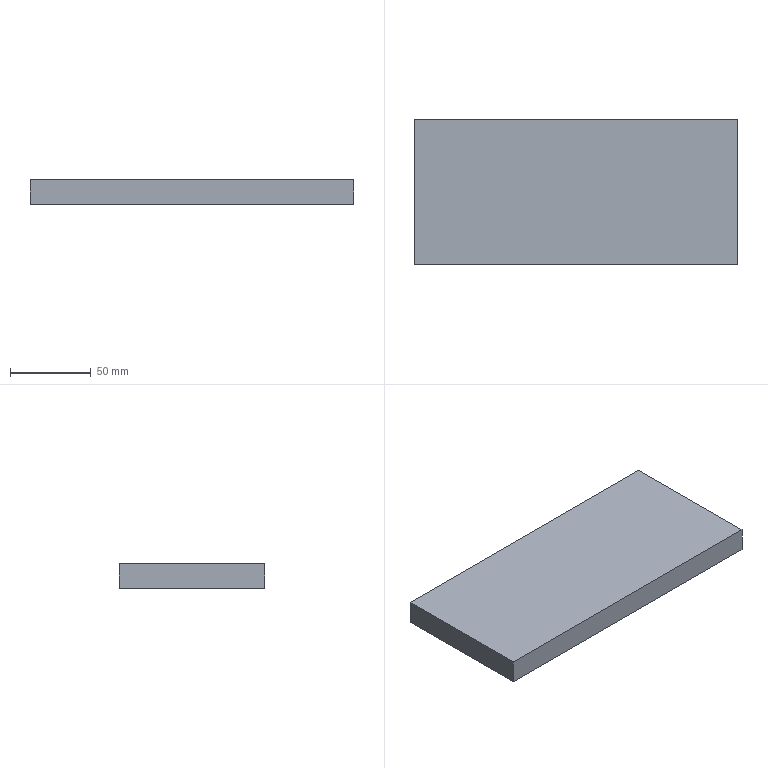Part | SolidWorks | features Extrusion 1 | 1 solid | 6 faces | box 200 x 90 x 15 mm | volume 270000 mm3 | plane 6
STEP:
#1=CARTESIAN_POINT('',(-100.,45.,-7.5));
#2=VERTEX_POINT('',#1);
#3=CARTESIAN_POINT('',(-100.,-45.,-7.5));
#4=VERTEX_POINT('',#3);
#5=CARTESIAN_POINT('',(-100.,-45.,-7.5));
#6=DIRECTION('',(0.,-1.,0.));
#7=VECTOR('',#6,1000.);
#8=LINE('',#5,#7);
#9=EDGE_CURVE('',#2,#4,#8,.T.);
#10=ORIENTED_EDGE('',*,*,#9,.T.);
#11=CARTESIAN_POINT('',(-100.,-45.,7.5));
#12=VERTEX_POINT('',#11);
#13=CARTESIAN_POINT('',(-100.,-45.,7.5));
#14=DIRECTION('',(0.,0.,-1.));
#15=VECTOR('',#14,1000.);
#16=LINE('',#13,#15);
#17=EDGE_CURVE('',#12,#4,#16,.T.);
#18=ORIENTED_EDGE('',*,*,#17,.F.);
#19=CARTESIAN_POINT('',(-100.,45.,7.5));
#20=VERTEX_POINT('',#19);
#21=CARTESIAN_POINT('',(-100.,-45.,7.5));
#22=DIRECTION('',(0.,-1.,0.));
#23=VECTOR('',#22,1000.);
#24=LINE('',#21,#23);
#25=EDGE_CURVE('',#20,#12,#24,.T.);
#26=ORIENTED_EDGE('',*,*,#25,.F.);
#27=CARTESIAN_POINT('',(-100.,45.,7.5));
#28=DIRECTION('',(0.,0.,-1.));
#29=VECTOR('',#28,1000.);
#30=LINE('',#27,#29);
#31=EDGE_CURVE('',#20,#2,#30,.T.);
#32=ORIENTED_EDGE('',*,*,#31,.T.);
#33=EDGE_LOOP('',(#10,#18,#26,#32));
#34=FACE_OUTER_BOUND('',#33,.T.);
#35=CARTESIAN_POINT('',(-100.,-45.,7.5));
#36=DIRECTION('',(1.,0.,0.));
#37=DIRECTION('',(0.,0.,-1.));
#38=AXIS2_PLACEMENT_3D('',#35,#36,#37);
#39=PLANE('',#38);
#40=ADVANCED_FACE('',(#34),#39,.F.);
#41=CARTESIAN_POINT('',(100.,-45.,-7.5));
#42=VERTEX_POINT('',#41);
#43=CARTESIAN_POINT('',(100.,-45.,-7.5));
#44=DIRECTION('',(1.,0.,0.));
#45=VECTOR('',#44,1000.);
#46=LINE('',#43,#45);
#47=EDGE_CURVE('',#4,#42,#46,.T.);
#48=ORIENTED_EDGE('',*,*,#47,.T.);
#49=CARTESIAN_POINT('',(100.,-45.,7.5));
#50=VERTEX_POINT('',#49);
#51=CARTESIAN_POINT('',(100.,-45.,7.5));
#52=DIRECTION('',(0.,0.,-1.));
#53=VECTOR('',#52,1000.);
#54=LINE('',#51,#53);
#55=EDGE_CURVE('',#50,#42,#54,.T.);
#56=ORIENTED_EDGE('',*,*,#55,.F.);
#57=CARTESIAN_POINT('',(100.,-45.,7.5));
#58=DIRECTION('',(1.,0.,0.));
#59=VECTOR('',#58,1000.);
#60=LINE('',#57,#59);
#61=EDGE_CURVE('',#12,#50,#60,.T.);
#62=ORIENTED_EDGE('',*,*,#61,.F.);
#63=ORIENTED_EDGE('',*,*,#17,.T.);
#64=EDGE_LOOP('',(#48,#56,#62,#63));
#65=FACE_OUTER_BOUND('',#64,.T.);
#66=CARTESIAN_POINT('',(100.,-45.,7.5));
#67=DIRECTION('',(0.,1.,0.));
#68=DIRECTION('',(-1.,0.,0.));
#69=AXIS2_PLACEMENT_3D('',#66,#67,#68);
#70=PLANE('',#69);
#71=ADVANCED_FACE('',(#65),#70,.F.);
#72=CARTESIAN_POINT('',(100.,45.,-7.5));
#73=VERTEX_POINT('',#72);
#74=CARTESIAN_POINT('',(100.,-45.,-7.5));
#75=DIRECTION('',(0.,1.,0.));
#76=VECTOR('',#75,1000.);
#77=LINE('',#74,#76);
#78=EDGE_CURVE('',#42,#73,#77,.T.);
#79=ORIENTED_EDGE('',*,*,#78,.T.);
#80=CARTESIAN_POINT('',(100.,45.,7.5));
#81=VERTEX_POINT('',#80);
#82=CARTESIAN_POINT('',(100.,45.,7.5));
#83=DIRECTION('',(0.,0.,-1.));
#84=VECTOR('',#83,1000.);
#85=LINE('',#82,#84);
#86=EDGE_CURVE('',#81,#73,#85,.T.);
#87=ORIENTED_EDGE('',*,*,#86,.F.);
#88=CARTESIAN_POINT('',(100.,-45.,7.5));
#89=DIRECTION('',(0.,1.,0.));
#90=VECTOR('',#89,1000.);
#91=LINE('',#88,#90);
#92=EDGE_CURVE('',#50,#81,#91,.T.);
#93=ORIENTED_EDGE('',*,*,#92,.F.);
#94=ORIENTED_EDGE('',*,*,#55,.T.);
#95=EDGE_LOOP('',(#79,#87,#93,#94));
#96=FACE_OUTER_BOUND('',#95,.T.);
#97=CARTESIAN_POINT('',(100.,-45.,7.5));
#98=DIRECTION('',(-1.,0.,0.));
#99=DIRECTION('',(0.,0.,1.));
#100=AXIS2_PLACEMENT_3D('',#97,#98,#99);
#101=PLANE('',#100);
#102=ADVANCED_FACE('',(#96),#101,.F.);
#103=CARTESIAN_POINT('',(100.,45.,-7.5));
#104=DIRECTION('',(-1.,0.,0.));
#105=VECTOR('',#104,1000.);
#106=LINE('',#103,#105);
#107=EDGE_CURVE('',#73,#2,#106,.T.);
#108=ORIENTED_EDGE('',*,*,#107,.T.);
#109=ORIENTED_EDGE('',*,*,#31,.F.);
#110=CARTESIAN_POINT('',(100.,45.,7.5));
#111=DIRECTION('',(-1.,0.,0.));
#112=VECTOR('',#111,1000.);
#113=LINE('',#110,#112);
#114=EDGE_CURVE('',#81,#20,#113,.T.);
#115=ORIENTED_EDGE('',*,*,#114,.F.);
#116=ORIENTED_EDGE('',*,*,#86,.T.);
#117=EDGE_LOOP('',(#108,#109,#115,#116));
#118=FACE_OUTER_BOUND('',#117,.T.);
#119=CARTESIAN_POINT('',(100.,45.,7.5));
#120=DIRECTION('',(0.,-1.,0.));
#121=DIRECTION('',(1.,0.,0.));
#122=AXIS2_PLACEMENT_3D('',#119,#120,#121);
#123=PLANE('',#122);
#124=ADVANCED_FACE('',(#118),#123,.F.);
#125=ORIENTED_EDGE('',*,*,#25,.T.);
#126=ORIENTED_EDGE('',*,*,#61,.T.);
#127=ORIENTED_EDGE('',*,*,#92,.T.);
#128=ORIENTED_EDGE('',*,*,#114,.T.);
#129=EDGE_LOOP('',(#125,#126,#127,#128));
#130=FACE_OUTER_BOUND('',#129,.T.);
#131=CARTESIAN_POINT('',(0.,0.,7.5));
#132=DIRECTION('',(0.,0.,1.));
#133=DIRECTION('',(1.,0.,0.));
#134=AXIS2_PLACEMENT_3D('',#131,#132,#133);
#135=PLANE('',#134);
#136=ADVANCED_FACE('',(#130),#135,.T.);
#137=ORIENTED_EDGE('',*,*,#9,.F.);
#138=ORIENTED_EDGE('',*,*,#107,.F.);
#139=ORIENTED_EDGE('',*,*,#78,.F.);
#140=ORIENTED_EDGE('',*,*,#47,.F.);
#141=EDGE_LOOP('',(#137,#138,#139,#140));
#142=FACE_OUTER_BOUND('',#141,.T.);
#143=CARTESIAN_POINT('',(0.,0.,-7.5));
#144=DIRECTION('',(0.,0.,1.));
#145=DIRECTION('',(1.,0.,0.));
#146=AXIS2_PLACEMENT_3D('',#143,#144,#145);
#147=PLANE('',#146);
#148=ADVANCED_FACE('',(#142),#147,.F.);
#149=CLOSED_SHELL('',(#40,#71,#102,#124,#136,#148));
#150=MANIFOLD_SOLID_BREP('',#149);
#151=CARTESIAN_POINT('',(0.,0.,0.));
#152=DIRECTION('',(0.,0.,1.));
#153=DIRECTION('',(1.,0.,0.));
#154=AXIS2_PLACEMENT_3D('',#151,#152,#153);
#155=(LENGTH_UNIT()NAMED_UNIT(*)SI_UNIT(.MILLI.,.METRE.));
#156=UNCERTAINTY_MEASURE_WITH_UNIT(LENGTH_MEASURE(0.00001),#155,'','');
#157=(NAMED_UNIT(*)PLANE_ANGLE_UNIT()SI_UNIT($,.RADIAN.));
#158=(NAMED_UNIT(*)SI_UNIT($,.STERADIAN.)SOLID_ANGLE_UNIT());
#159=(GEOMETRIC_REPRESENTATION_CONTEXT(3)GLOBAL_UNCERTAINTY_ASSIGNED_CONTEXT((#156))GLOBAL_UNIT_ASSIGNED_CONTEXT((#155,#157,#158))REPRESENTATION_CONTEXT('',''));
#160=ADVANCED_BREP_SHAPE_REPRESENTATION('',(#150,#154),#159);